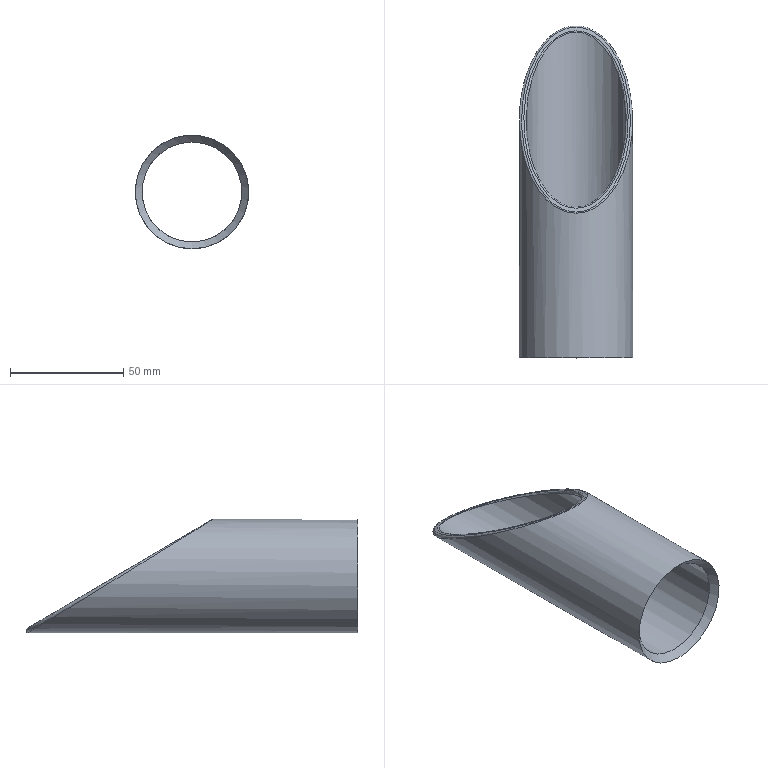Part | STEP file | JBJ-P-1004-05 | 1 solid | 6 faces | box 50 x 146.328 x 50 mm | volume 46289 mm3 | cylinder 2 | spline 2 | plane 1 | cone 1 | commonest cylinder face diameters 44 x1 50 x1
STEP:
#1=CARTESIAN_POINT('',(0.,1.,-25.));
#2=VERTEX_POINT('',#1);
#3=CARTESIAN_POINT('',(0.,1.,0.));
#4=DIRECTION('',(0.,1.,0.));
#5=DIRECTION('',(0.,0.,-1.));
#6=AXIS2_PLACEMENT_3D('',#3,#4,#5);
#7=CIRCLE('',#6,25.);
#8=EDGE_CURVE('',#2,#2,#7,.T.);
#9=ORIENTED_EDGE('',*,*,#8,.T.);
#10=EDGE_LOOP('',(#9));
#11=FACE_OUTER_BOUND('',#10,.T.);
#12=CARTESIAN_POINT('',(0.,64.728,25.));
#13=VERTEX_POINT('',#12);
#14=CARTESIAN_POINT('',(0.,64.728,25.));
#15=CARTESIAN_POINT('',(-50.,64.728,25.));
#16=CARTESIAN_POINT('',(-50.,146.328,-25.));
#17=CARTESIAN_POINT('',(0.,146.328,-25.));
#18=CARTESIAN_POINT('',(50.,146.328,-25.));
#19=CARTESIAN_POINT('',(50.,64.728,25.));
#20=CARTESIAN_POINT('',(0.,64.728,25.));
#21=(BOUNDED_CURVE()B_SPLINE_CURVE(3,(#14,#15,#16,#17,#18,#19,#20),.UNSPECIFIED.,.T.,.T.)B_SPLINE_CURVE_WITH_KNOTS((4,3,4),(0.,3.142,6.283),.UNSPECIFIED.)CURVE()GEOMETRIC_REPRESENTATION_ITEM()RATIONAL_B_SPLINE_CURVE((1.,0.3333,0.3333,1.,0.3333,0.3333,1.))REPRESENTATION_ITEM(''));
#22=EDGE_CURVE('',#13,#13,#21,.T.);
#23=ORIENTED_EDGE('',*,*,#22,.T.);
#24=EDGE_LOOP('',(#23));
#25=FACE_OUTER_BOUND('',#24,.T.);
#26=CARTESIAN_POINT('',(0.,150.,0.));
#27=DIRECTION('',(0.,-1.,0.));
#28=DIRECTION('',(0.,0.,-1.));
#29=AXIS2_PLACEMENT_3D('',#26,#27,#28);
#30=CYLINDRICAL_SURFACE('',#29,25.);
#31=ADVANCED_FACE('',(#11,#25),#30,.T.);
#32=CARTESIAN_POINT('',(0.,4.,22.));
#33=VERTEX_POINT('',#32);
#34=CARTESIAN_POINT('',(0.,4.,0.));
#35=DIRECTION('',(0.,-1.,0.));
#36=DIRECTION('',(0.,0.,1.));
#37=AXIS2_PLACEMENT_3D('',#34,#35,#36);
#38=CIRCLE('',#37,22.);
#39=EDGE_CURVE('',#33,#33,#38,.T.);
#40=ORIENTED_EDGE('',*,*,#39,.T.);
#41=EDGE_LOOP('',(#40));
#42=FACE_OUTER_BOUND('',#41,.T.);
#43=CARTESIAN_POINT('',(0.,66.428,22.));
#44=VERTEX_POINT('',#43);
#45=CARTESIAN_POINT('',(0.,66.428,22.));
#46=CARTESIAN_POINT('',(44.,66.428,22.));
#47=CARTESIAN_POINT('',(44.,144.628,-22.));
#48=CARTESIAN_POINT('',(0.,144.628,-22.));
#49=CARTESIAN_POINT('',(-44.,144.628,-22.));
#50=CARTESIAN_POINT('',(-44.,66.428,22.));
#51=CARTESIAN_POINT('',(0.,66.428,22.));
#52=(BOUNDED_CURVE()B_SPLINE_CURVE(3,(#45,#46,#47,#48,#49,#50,#51),.UNSPECIFIED.,.T.,.F.)B_SPLINE_CURVE_WITH_KNOTS((4,3,4),(0.,3.142,6.283),.UNSPECIFIED.)CURVE()GEOMETRIC_REPRESENTATION_ITEM()RATIONAL_B_SPLINE_CURVE((1.,0.3333,0.3333,1.,0.3333,0.3333,1.))REPRESENTATION_ITEM(''));
#53=EDGE_CURVE('',#44,#44,#52,.T.);
#54=ORIENTED_EDGE('',*,*,#53,.T.);
#55=EDGE_LOOP('',(#54));
#56=FACE_OUTER_BOUND('',#55,.T.);
#57=CARTESIAN_POINT('',(0.,150.,0.));
#58=DIRECTION('',(0.,-1.,0.));
#59=DIRECTION('',(0.,0.,-1.));
#60=AXIS2_PLACEMENT_3D('',#57,#58,#59);
#61=CYLINDRICAL_SURFACE('',#60,22.);
#62=ADVANCED_FACE('',(#42,#56),#61,.F.);
#63=CARTESIAN_POINT('',(0.,66.935,23.862));
#64=VERTEX_POINT('',#63);
#65=CARTESIAN_POINT('',(0.,66.935,23.862));
#66=CARTESIAN_POINT('',(-46.,66.935,23.862));
#67=CARTESIAN_POINT('',(-46.,145.135,-22.138));
#68=CARTESIAN_POINT('',(0.,145.135,-22.138));
#69=CARTESIAN_POINT('',(46.,145.135,-22.138));
#70=CARTESIAN_POINT('',(46.,66.935,23.862));
#71=CARTESIAN_POINT('',(0.,66.935,23.862));
#72=(BOUNDED_CURVE()B_SPLINE_CURVE(3,(#65,#66,#67,#68,#69,#70,#71),.UNSPECIFIED.,.T.,.F.)B_SPLINE_CURVE_WITH_KNOTS((4,3,4),(0.,3.142,6.283),.UNSPECIFIED.)CURVE()GEOMETRIC_REPRESENTATION_ITEM()RATIONAL_B_SPLINE_CURVE((1.,0.3333,0.3333,1.,0.3333,0.3333,1.))REPRESENTATION_ITEM(''));
#73=EDGE_CURVE('',#64,#64,#72,.T.);
#74=ORIENTED_EDGE('',*,*,#73,.T.);
#75=EDGE_LOOP('',(#74));
#76=FACE_BOUND('',#75,.T.);
#77=CARTESIAN_POINT('',(0.,65.235,24.862));
#78=VERTEX_POINT('',#77);
#79=CARTESIAN_POINT('',(0.,65.235,24.862));
#80=CARTESIAN_POINT('',(48.,65.235,24.862));
#81=CARTESIAN_POINT('',(48.,146.835,-23.138));
#82=CARTESIAN_POINT('',(0.,146.835,-23.138));
#83=CARTESIAN_POINT('',(-48.,146.835,-23.138));
#84=CARTESIAN_POINT('',(-48.,65.235,24.862));
#85=CARTESIAN_POINT('',(0.,65.235,24.862));
#86=(BOUNDED_CURVE()B_SPLINE_CURVE(3,(#79,#80,#81,#82,#83,#84,#85),.UNSPECIFIED.,.T.,.F.)B_SPLINE_CURVE_WITH_KNOTS((4,3,4),(0.,3.142,6.283),.UNSPECIFIED.)CURVE()GEOMETRIC_REPRESENTATION_ITEM()RATIONAL_B_SPLINE_CURVE((1.,0.3333,0.3333,1.,0.3333,0.3333,1.))REPRESENTATION_ITEM(''));
#87=EDGE_CURVE('',#78,#78,#86,.T.);
#88=ORIENTED_EDGE('',*,*,#87,.T.);
#89=EDGE_LOOP('',(#88));
#90=FACE_OUTER_BOUND('',#89,.T.);
#91=CARTESIAN_POINT('',(-25.,65.,25.));
#92=DIRECTION('',(0.,-0.507,-0.8619));
#93=DIRECTION('',(0.,0.8619,-0.507));
#94=AXIS2_PLACEMENT_3D('',#91,#92,#93);
#95=PLANE('',#94);
#96=ADVANCED_FACE('',(#76,#90),#95,.F.);
#97=ORIENTED_EDGE('',*,*,#53,.F.);
#98=EDGE_LOOP('',(#97));
#99=FACE_OUTER_BOUND('',#98,.T.);
#100=ORIENTED_EDGE('',*,*,#73,.F.);
#101=EDGE_LOOP('',(#100));
#102=FACE_OUTER_BOUND('',#101,.T.);
#103=CARTESIAN_POINT('',(0.,66.428,22.));
#104=CARTESIAN_POINT('',(0.,70.1,22.));
#105=CARTESIAN_POINT('',(0.,66.935,23.862));
#106=CARTESIAN_POINT('',(-0.7199,66.428,22.));
#107=CARTESIAN_POINT('',(-0.5156,70.1,22.));
#108=CARTESIAN_POINT('',(-0.7527,66.935,23.862));
#109=CARTESIAN_POINT('',(-1.44,66.491,21.965));
#110=CARTESIAN_POINT('',(-1.026,70.124,21.986));
#111=CARTESIAN_POINT('',(-1.505,66.998,23.825));
#112=CARTESIAN_POINT('',(-2.873,66.741,21.823));
#113=CARTESIAN_POINT('',(-2.093,70.237,21.92));
#114=CARTESIAN_POINT('',(-3.003,67.248,23.677));
#115=CARTESIAN_POINT('',(-3.586,66.929,21.718));
#116=CARTESIAN_POINT('',(-2.639,70.323,21.869));
#117=CARTESIAN_POINT('',(-3.749,67.436,23.567));
#118=CARTESIAN_POINT('',(-4.998,67.429,21.437));
#119=CARTESIAN_POINT('',(-3.791,70.589,21.713));
#120=CARTESIAN_POINT('',(-5.225,67.936,23.273));
#121=CARTESIAN_POINT('',(-5.697,67.74,21.262));
#122=CARTESIAN_POINT('',(-4.386,70.764,21.61));
#123=CARTESIAN_POINT('',(-5.956,68.247,23.09));
#124=CARTESIAN_POINT('',(-7.075,68.483,20.844));
#125=CARTESIAN_POINT('',(-5.624,71.236,21.332));
#126=CARTESIAN_POINT('',(-7.397,68.99,22.653));
#127=CARTESIAN_POINT('',(-7.754,68.914,20.601));
#128=CARTESIAN_POINT('',(-6.259,71.526,21.161));
#129=CARTESIAN_POINT('',(-8.106,69.421,22.399));
#130=CARTESIAN_POINT('',(-9.084,69.894,20.05));
#131=CARTESIAN_POINT('',(-7.553,72.242,20.74));
#132=CARTESIAN_POINT('',(-9.497,70.401,21.823));
#133=CARTESIAN_POINT('',(-9.736,70.441,19.742));
#134=CARTESIAN_POINT('',(-8.206,72.659,20.495));
#135=CARTESIAN_POINT('',(-10.178,70.948,21.501));
#136=CARTESIAN_POINT('',(-11.006,71.648,19.063));
#137=CARTESIAN_POINT('',(-9.512,73.631,19.923));
#138=CARTESIAN_POINT('',(-11.506,72.155,20.791));
#139=CARTESIAN_POINT('',(-11.624,72.306,18.692));
#140=CARTESIAN_POINT('',(-10.161,74.177,19.602));
#141=CARTESIAN_POINT('',(-12.152,72.813,20.404));
#142=CARTESIAN_POINT('',(-13.42,74.439,17.492));
#143=CARTESIAN_POINT('',(-12.027,75.966,18.549));
#144=CARTESIAN_POINT('',(-14.03,74.946,19.149));
#145=CARTESIAN_POINT('',(-14.538,76.07,16.575));
#146=CARTESIAN_POINT('',(-13.261,77.411,17.699));
#147=CARTESIAN_POINT('',(-15.199,76.577,18.19));
#148=CARTESIAN_POINT('',(-16.575,79.689,14.538));
#149=CARTESIAN_POINT('',(-15.529,80.774,15.721));
#150=CARTESIAN_POINT('',(-17.328,80.196,16.061));
#151=CARTESIAN_POINT('',(-17.492,81.677,13.42));
#152=CARTESIAN_POINT('',(-16.575,82.641,14.623));
#153=CARTESIAN_POINT('',(-18.287,82.184,14.892));
#154=CARTESIAN_POINT('',(-19.092,85.933,11.025));
#155=CARTESIAN_POINT('',(-18.399,86.73,12.218));
#156=CARTESIAN_POINT('',(-19.96,86.44,12.388));
#157=CARTESIAN_POINT('',(-19.774,88.2,9.749));
#158=CARTESIAN_POINT('',(-19.199,88.923,10.928));
#159=CARTESIAN_POINT('',(-20.673,88.707,11.054));
#160=CARTESIAN_POINT('',(-20.876,92.929,7.089));
#161=CARTESIAN_POINT('',(-20.492,93.54,8.211));
#162=CARTESIAN_POINT('',(-21.825,93.436,8.273));
#163=CARTESIAN_POINT('',(-21.296,95.39,5.704));
#164=CARTESIAN_POINT('',(-21.01,95.955,6.791));
#165=CARTESIAN_POINT('',(-22.264,95.897,6.825));
#166=CARTESIAN_POINT('',(-21.858,100.41,2.88));
#167=CARTESIAN_POINT('',(-21.724,100.899,3.883));
#168=CARTESIAN_POINT('',(-22.852,100.917,3.873));
#169=CARTESIAN_POINT('',(-22.,102.969,1.44));
#170=CARTESIAN_POINT('',(-21.942,103.431,2.394));
#171=CARTESIAN_POINT('',(-23.,103.476,2.367));
#172=CARTESIAN_POINT('',(-22.,108.087,-1.44));
#173=CARTESIAN_POINT('',(-22.055,108.496,-0.5858));
#174=CARTESIAN_POINT('',(-23.,108.594,-0.6434));
#175=CARTESIAN_POINT('',(-21.858,110.646,-2.88));
#176=CARTESIAN_POINT('',(-21.967,111.04,-2.082));
#177=CARTESIAN_POINT('',(-22.852,111.153,-2.149));
#178=CARTESIAN_POINT('',(-21.296,115.666,-5.704));
#179=CARTESIAN_POINT('',(-21.481,116.022,-5.013));
#180=CARTESIAN_POINT('',(-22.264,116.173,-5.102));
#181=CARTESIAN_POINT('',(-20.876,118.126,-7.089));
#182=CARTESIAN_POINT('',(-21.095,118.476,-6.456));
#183=CARTESIAN_POINT('',(-21.825,118.633,-6.549));
#184=CARTESIAN_POINT('',(-19.774,122.855,-9.749));
#185=CARTESIAN_POINT('',(-20.035,123.176,-9.221));
#186=CARTESIAN_POINT('',(-20.673,123.362,-9.331));
#187=CARTESIAN_POINT('',(-19.092,125.123,-11.025));
#188=CARTESIAN_POINT('',(-19.368,125.442,-10.554));
#189=CARTESIAN_POINT('',(-19.96,125.63,-10.665));
#190=CARTESIAN_POINT('',(-17.492,129.378,-13.42));
#191=CARTESIAN_POINT('',(-17.78,129.677,-13.045));
#192=CARTESIAN_POINT('',(-18.287,129.885,-13.168));
#193=CARTESIAN_POINT('',(-16.575,131.366,-14.538));
#194=CARTESIAN_POINT('',(-16.862,131.666,-14.215));
#195=CARTESIAN_POINT('',(-17.328,131.873,-14.337));
#196=CARTESIAN_POINT('',(-14.538,134.985,-16.575));
#197=CARTESIAN_POINT('',(-14.812,135.27,-16.335));
#198=CARTESIAN_POINT('',(-15.199,135.492,-16.466));
#199=CARTESIAN_POINT('',(-13.42,136.616,-17.492));
#200=CARTESIAN_POINT('',(-13.68,136.904,-17.297));
#201=CARTESIAN_POINT('',(-14.03,137.123,-17.426));
#202=CARTESIAN_POINT('',(-11.025,139.46,-19.092));
#203=CARTESIAN_POINT('',(-11.251,139.737,-18.963));
#204=CARTESIAN_POINT('',(-11.526,139.967,-19.098));
#205=CARTESIAN_POINT('',(-9.749,140.672,-19.774));
#206=CARTESIAN_POINT('',(-9.951,140.952,-19.678));
#207=CARTESIAN_POINT('',(-10.192,141.179,-19.811));
#208=CARTESIAN_POINT('',(-7.089,142.631,-20.876));
#209=CARTESIAN_POINT('',(-7.242,142.904,-20.826));
#210=CARTESIAN_POINT('',(-7.411,143.138,-20.963));
#211=CARTESIAN_POINT('',(-5.704,143.377,-21.296));
#212=CARTESIAN_POINT('',(-5.827,143.652,-21.266));
#213=CARTESIAN_POINT('',(-5.963,143.884,-21.402));
#214=CARTESIAN_POINT('',(-2.88,144.376,-21.858));
#215=CARTESIAN_POINT('',(-2.945,144.647,-21.851));
#216=CARTESIAN_POINT('',(-3.011,144.883,-21.99));
#217=CARTESIAN_POINT('',(-1.44,144.628,-22.));
#218=CARTESIAN_POINT('',(-1.47,144.9,-22.));
#219=CARTESIAN_POINT('',(-1.505,145.135,-22.138));
#220=CARTESIAN_POINT('',(1.44,144.628,-22.));
#221=CARTESIAN_POINT('',(1.47,144.9,-22.));
#222=CARTESIAN_POINT('',(1.505,145.135,-22.138));
#223=CARTESIAN_POINT('',(2.88,144.376,-21.858));
#224=CARTESIAN_POINT('',(2.945,144.647,-21.851));
#225=CARTESIAN_POINT('',(3.011,144.883,-21.99));
#226=CARTESIAN_POINT('',(5.704,143.377,-21.296));
#227=CARTESIAN_POINT('',(5.827,143.652,-21.266));
#228=CARTESIAN_POINT('',(5.963,143.884,-21.402));
#229=CARTESIAN_POINT('',(7.089,142.631,-20.876));
#230=CARTESIAN_POINT('',(7.242,142.904,-20.826));
#231=CARTESIAN_POINT('',(7.411,143.138,-20.963));
#232=CARTESIAN_POINT('',(9.749,140.672,-19.774));
#233=CARTESIAN_POINT('',(9.951,140.952,-19.678));
#234=CARTESIAN_POINT('',(10.192,141.179,-19.811));
#235=CARTESIAN_POINT('',(11.025,139.46,-19.092));
#236=CARTESIAN_POINT('',(11.251,139.737,-18.963));
#237=CARTESIAN_POINT('',(11.526,139.967,-19.098));
#238=CARTESIAN_POINT('',(13.42,136.616,-17.492));
#239=CARTESIAN_POINT('',(13.68,136.904,-17.297));
#240=CARTESIAN_POINT('',(14.03,137.123,-17.426));
#241=CARTESIAN_POINT('',(14.538,134.985,-16.575));
#242=CARTESIAN_POINT('',(14.812,135.27,-16.335));
#243=CARTESIAN_POINT('',(15.199,135.492,-16.466));
#244=CARTESIAN_POINT('',(16.575,131.366,-14.538));
#245=CARTESIAN_POINT('',(16.862,131.666,-14.215));
#246=CARTESIAN_POINT('',(17.328,131.873,-14.337));
#247=CARTESIAN_POINT('',(17.492,129.378,-13.42));
#248=CARTESIAN_POINT('',(17.78,129.677,-13.045));
#249=CARTESIAN_POINT('',(18.287,129.885,-13.168));
#250=CARTESIAN_POINT('',(19.092,125.123,-11.025));
#251=CARTESIAN_POINT('',(19.368,125.442,-10.554));
#252=CARTESIAN_POINT('',(19.96,125.63,-10.665));
#253=CARTESIAN_POINT('',(19.774,122.855,-9.749));
#254=CARTESIAN_POINT('',(20.035,123.176,-9.221));
#255=CARTESIAN_POINT('',(20.673,123.362,-9.331));
#256=CARTESIAN_POINT('',(20.876,118.126,-7.089));
#257=CARTESIAN_POINT('',(21.095,118.476,-6.456));
#258=CARTESIAN_POINT('',(21.825,118.633,-6.549));
#259=CARTESIAN_POINT('',(21.296,115.666,-5.704));
#260=CARTESIAN_POINT('',(21.481,116.022,-5.013));
#261=CARTESIAN_POINT('',(22.264,116.173,-5.102));
#262=CARTESIAN_POINT('',(21.858,110.646,-2.88));
#263=CARTESIAN_POINT('',(21.967,111.04,-2.082));
#264=CARTESIAN_POINT('',(22.852,111.153,-2.149));
#265=CARTESIAN_POINT('',(22.,108.087,-1.44));
#266=CARTESIAN_POINT('',(22.055,108.496,-0.5858));
#267=CARTESIAN_POINT('',(23.,108.594,-0.6434));
#268=CARTESIAN_POINT('',(22.,102.969,1.44));
#269=CARTESIAN_POINT('',(21.942,103.431,2.394));
#270=CARTESIAN_POINT('',(23.,103.476,2.367));
#271=CARTESIAN_POINT('',(21.858,100.41,2.88));
#272=CARTESIAN_POINT('',(21.724,100.899,3.883));
#273=CARTESIAN_POINT('',(22.852,100.917,3.873));
#274=CARTESIAN_POINT('',(21.296,95.39,5.704));
#275=CARTESIAN_POINT('',(21.01,95.955,6.791));
#276=CARTESIAN_POINT('',(22.264,95.897,6.825));
#277=CARTESIAN_POINT('',(20.876,92.929,7.089));
#278=CARTESIAN_POINT('',(20.492,93.54,8.211));
#279=CARTESIAN_POINT('',(21.825,93.436,8.273));
#280=CARTESIAN_POINT('',(19.774,88.2,9.749));
#281=CARTESIAN_POINT('',(19.199,88.923,10.928));
#282=CARTESIAN_POINT('',(20.673,88.707,11.054));
#283=CARTESIAN_POINT('',(19.092,85.933,11.025));
#284=CARTESIAN_POINT('',(18.399,86.73,12.218));
#285=CARTESIAN_POINT('',(19.96,86.44,12.388));
#286=CARTESIAN_POINT('',(17.492,81.677,13.42));
#287=CARTESIAN_POINT('',(16.575,82.641,14.623));
#288=CARTESIAN_POINT('',(18.287,82.184,14.892));
#289=CARTESIAN_POINT('',(16.575,79.689,14.538));
#290=CARTESIAN_POINT('',(15.529,80.774,15.721));
#291=CARTESIAN_POINT('',(17.328,80.196,16.061));
#292=CARTESIAN_POINT('',(14.538,76.07,16.575));
#293=CARTESIAN_POINT('',(13.261,77.411,17.699));
#294=CARTESIAN_POINT('',(15.199,76.577,18.19));
#295=CARTESIAN_POINT('',(13.42,74.439,17.492));
#296=CARTESIAN_POINT('',(12.027,75.966,18.549));
#297=CARTESIAN_POINT('',(14.03,74.946,19.149));
#298=CARTESIAN_POINT('',(11.624,72.306,18.692));
#299=CARTESIAN_POINT('',(10.161,74.177,19.602));
#300=CARTESIAN_POINT('',(12.152,72.813,20.404));
#301=CARTESIAN_POINT('',(11.006,71.648,19.063));
#302=CARTESIAN_POINT('',(9.512,73.631,19.923));
#303=CARTESIAN_POINT('',(11.506,72.155,20.791));
#304=CARTESIAN_POINT('',(9.736,70.441,19.742));
#305=CARTESIAN_POINT('',(8.206,72.659,20.495));
#306=CARTESIAN_POINT('',(10.178,70.948,21.501));
#307=CARTESIAN_POINT('',(9.084,69.894,20.05));
#308=CARTESIAN_POINT('',(7.553,72.242,20.74));
#309=CARTESIAN_POINT('',(9.497,70.401,21.823));
#310=CARTESIAN_POINT('',(7.754,68.914,20.601));
#311=CARTESIAN_POINT('',(6.259,71.526,21.161));
#312=CARTESIAN_POINT('',(8.106,69.421,22.399));
#313=CARTESIAN_POINT('',(7.075,68.483,20.844));
#314=CARTESIAN_POINT('',(5.624,71.236,21.332));
#315=CARTESIAN_POINT('',(7.397,68.99,22.653));
#316=CARTESIAN_POINT('',(5.697,67.74,21.262));
#317=CARTESIAN_POINT('',(4.386,70.764,21.61));
#318=CARTESIAN_POINT('',(5.956,68.247,23.09));
#319=CARTESIAN_POINT('',(4.998,67.429,21.437));
#320=CARTESIAN_POINT('',(3.791,70.589,21.713));
#321=CARTESIAN_POINT('',(5.225,67.936,23.273));
#322=CARTESIAN_POINT('',(3.586,66.929,21.718));
#323=CARTESIAN_POINT('',(2.639,70.323,21.869));
#324=CARTESIAN_POINT('',(3.749,67.436,23.567));
#325=CARTESIAN_POINT('',(2.873,66.741,21.823));
#326=CARTESIAN_POINT('',(2.093,70.237,21.92));
#327=CARTESIAN_POINT('',(3.003,67.248,23.677));
#328=CARTESIAN_POINT('',(1.44,66.491,21.965));
#329=CARTESIAN_POINT('',(1.026,70.124,21.986));
#330=CARTESIAN_POINT('',(1.505,66.998,23.825));
#331=CARTESIAN_POINT('',(0.7199,66.428,22.));
#332=CARTESIAN_POINT('',(0.5156,70.1,22.));
#333=CARTESIAN_POINT('',(0.7527,66.935,23.862));
#334=CARTESIAN_POINT('',(0.,66.428,22.));
#335=CARTESIAN_POINT('',(0.,70.1,22.));
#336=CARTESIAN_POINT('',(0.,66.935,23.862));
#337=(BOUNDED_SURFACE()B_SPLINE_SURFACE(3,2,((#103,#104,#105),(#106,#107,#108),(#109,#110,#111),(#112,#113,#114),(#115,#116,#117),(#118,#119,#120),(#121,#122,#123),(#124,#125,#126),(#127,#128,#129),(#130,#131,#132),(#133,#134,#135),(#136,#137,#138),(#139,#140,#141),(#142,#143,#144),(#145,#146,#147),(#148,#149,#150),(#151,#152,#153),(#154,#155,#156),(#157,#158,#159),(#160,#161,#162),(#163,#164,#165),(#166,#167,#168),(#169,#170,#171),(#172,#173,#174),(#175,#176,#177),(#178,#179,#180),(#181,#182,#183),(#184,#185,#186),(#187,#188,#189),(#190,#191,#192),(#193,#194,#195),(#196,#197,#198),(#199,#200,#201),(#202,#203,#204),(#205,#206,#207),(#208,#209,#210),(#211,#212,#213),(#214,#215,#216),(#217,#218,#219),(#220,#221,#222),(#223,#224,#225),(#226,#227,#228),(#229,#230,#231),(#232,#233,#234),(#235,#236,#237),(#238,#239,#240),(#241,#242,#243),(#244,#245,#246),(#247,#248,#249),(#250,#251,#252),(#253,#254,#255),(#256,#257,#258),(#259,#260,#261),(#262,#263,#264),(#265,#266,#267),(#268,#269,#270),(#271,#272,#273),(#274,#275,#276),(#277,#278,#279),(#280,#281,#282),(#283,#284,#285),(#286,#287,#288),(#289,#290,#291),(#292,#293,#294),(#295,#296,#297),(#298,#299,#300),(#301,#302,#303),(#304,#305,#306),(#307,#308,#309),(#310,#311,#312),(#313,#314,#315),(#316,#317,#318),(#319,#320,#321),(#322,#323,#324),(#325,#326,#327),(#328,#329,#330),(#331,#332,#333),(#334,#335,#336)),.UNSPECIFIED.,.T.,.F.,.F.)B_SPLINE_SURFACE_WITH_KNOTS((4,2,2,2,2,2,2,2,2,2,2,2,2,2,2,2,2,2,2,2,2,2,2,2,2,2,2,2,2,2,2,2,2,2,2,2,2,2,4),(3,3),(0.,0.09817,0.1963,0.2945,0.3927,0.4909,0.589,0.7854,0.9817,1.178,1.374,1.571,1.767,1.963,2.16,2.356,2.553,2.749,2.945,3.142,3.338,3.534,3.731,3.927,4.123,4.32,4.516,4.712,4.909,5.105,5.301,5.498,5.694,5.792,5.89,5.989,6.087,6.185,6.283),(0.,1.),.UNSPECIFIED.)GEOMETRIC_REPRESENTATION_ITEM()RATIONAL_B_SPLINE_SURFACE(((1.,0.2627,1.),(1.,0.2627,1.),(1.,0.2641,1.),(1.,0.2693,1.),(1.,0.2731,1.),(1.,0.283,1.),(1.,0.289,1.),(1.,0.3029,1.),(1.,0.3107,1.),(1.,0.3276,1.),(1.,0.3367,1.),(1.,0.3559,1.),(1.,0.366,1.),(1.,0.3972,1.),(1.,0.4193,1.),(1.,0.4645,1.),(1.,0.4875,1.),(1.,0.5334,1.),(1.,0.5563,1.),(1.,0.6014,1.),(1.,0.6235,1.),(1.,0.6664,1.),(1.,0.6872,1.),(1.,0.7271,1.),(1.,0.7462,1.),(1.,0.7823,1.),(1.,0.7994,1.),(1.,0.8314,1.),(1.,0.8463,1.),(1.,0.8735,1.),(1.,0.886,1.),(1.,0.9082,1.),(1.,0.918,1.),(1.,0.9349,1.),(1.,0.942,1.),(1.,0.9534,1.),(1.,0.9577,1.),(1.,0.9634,1.),(1.,0.9649,1.),(1.,0.9649,1.),(1.,0.9634,1.),(1.,0.9577,1.),(1.,0.9534,1.),(1.,0.942,1.),(1.,0.9349,1.),(1.,0.918,1.),(1.,0.9082,1.),(1.,0.886,1.),(1.,0.8735,1.),(1.,0.8463,1.),(1.,0.8314,1.),(1.,0.7994,1.),(1.,0.7823,1.),(1.,0.7462,1.),(1.,0.7271,1.),(1.,0.6872,1.),(1.,0.6664,1.),(1.,0.6235,1.),(1.,0.6014,1.),(1.,0.5563,1.),(1.,0.5334,1.),(1.,0.4875,1.),(1.,0.4645,1.),(1.,0.4193,1.),(1.,0.3972,1.),(1.,0.366,1.),(1.,0.3559,1.),(1.,0.3367,1.),(1.,0.3276,1.),(1.,0.3107,1.),(1.,0.3029,1.),(1.,0.289,1.),(1.,0.283,1.),(1.,0.2731,1.),(1.,0.2693,1.),(1.,0.2641,1.),(1.,0.2627,1.),(1.,0.2627,1.)))REPRESENTATION_ITEM('')SURFACE());
#338=ADVANCED_FACE('',(#99,#102),#337,.T.);
#339=ORIENTED_EDGE('',*,*,#87,.F.);
#340=EDGE_LOOP('',(#339));
#341=FACE_OUTER_BOUND('',#340,.T.);
#342=ORIENTED_EDGE('',*,*,#22,.F.);
#343=EDGE_LOOP('',(#342));
#344=FACE_OUTER_BOUND('',#343,.T.);
#345=CARTESIAN_POINT('',(0.,65.235,24.862));
#346=CARTESIAN_POINT('',(0.,65.,25.));
#347=CARTESIAN_POINT('',(0.,64.728,25.));
#348=CARTESIAN_POINT('',(-1.571,65.235,24.862));
#349=CARTESIAN_POINT('',(-1.606,65.,25.));
#350=CARTESIAN_POINT('',(-1.636,64.728,25.));
#351=CARTESIAN_POINT('',(-3.142,65.498,24.707));
#352=CARTESIAN_POINT('',(-3.217,65.265,24.844));
#353=CARTESIAN_POINT('',(-3.272,64.991,24.839));
#354=CARTESIAN_POINT('',(-6.223,66.54,24.094));
#355=CARTESIAN_POINT('',(-6.369,66.311,24.229));
#356=CARTESIAN_POINT('',(-6.482,66.033,24.2));
#357=CARTESIAN_POINT('',(-7.733,67.319,23.636));
#358=CARTESIAN_POINT('',(-7.919,67.096,23.767));
#359=CARTESIAN_POINT('',(-8.055,66.812,23.723));
#360=CARTESIAN_POINT('',(-10.636,69.362,22.434));
#361=CARTESIAN_POINT('',(-10.894,69.147,22.56));
#362=CARTESIAN_POINT('',(-11.079,68.855,22.471));
#363=CARTESIAN_POINT('',(-12.028,70.627,21.69));
#364=CARTESIAN_POINT('',(-12.326,70.424,21.81));
#365=CARTESIAN_POINT('',(-12.529,70.12,21.696));
#366=CARTESIAN_POINT('',(-14.64,73.594,19.945));
#367=CARTESIAN_POINT('',(-15.013,73.402,20.058));
#368=CARTESIAN_POINT('',(-15.25,73.087,19.878));
#369=CARTESIAN_POINT('',(-15.86,75.297,18.943));
#370=CARTESIAN_POINT('',(-16.274,75.12,19.047));
#371=CARTESIAN_POINT('',(-16.521,74.79,18.835));
#372=CARTESIAN_POINT('',(-18.081,79.073,16.722));
#373=CARTESIAN_POINT('',(-18.575,78.913,16.816));
#374=CARTESIAN_POINT('',(-18.835,78.566,16.521));
#375=CARTESIAN_POINT('',(-19.083,81.147,15.502));
#376=CARTESIAN_POINT('',(-19.617,81.007,15.584));
#377=CARTESIAN_POINT('',(-19.878,80.64,15.25));
#378=CARTESIAN_POINT('',(-20.828,85.588,12.89));
#379=CARTESIAN_POINT('',(-21.447,85.47,12.959));
#380=CARTESIAN_POINT('',(-21.696,85.081,12.529));
#381=CARTESIAN_POINT('',(-21.572,87.954,11.498));
#382=CARTESIAN_POINT('',(-22.233,87.861,11.552));
#383=CARTESIAN_POINT('',(-22.471,87.447,11.079));
#384=CARTESIAN_POINT('',(-22.774,92.888,8.595));
#385=CARTESIAN_POINT('',(-23.528,92.827,8.631));
#386=CARTESIAN_POINT('',(-23.723,92.381,8.055));
#387=CARTESIAN_POINT('',(-23.232,95.456,7.085));
#388=CARTESIAN_POINT('',(-24.03,95.424,7.104));
#389=CARTESIAN_POINT('',(-24.2,94.949,6.482));
#390=CARTESIAN_POINT('',(-23.845,100.694,4.003));
#391=CARTESIAN_POINT('',(-24.744,100.706,3.997));
#392=CARTESIAN_POINT('',(-24.839,100.187,3.272));
#393=CARTESIAN_POINT('',(-24.,103.364,2.433));
#394=CARTESIAN_POINT('',(-24.945,103.41,2.406));
#395=CARTESIAN_POINT('',(-25.,102.857,1.636));
#396=CARTESIAN_POINT('',(-24.,108.705,-0.7089));
#397=CARTESIAN_POINT('',(-25.058,108.812,-0.7718));
#398=CARTESIAN_POINT('',(-25.,108.198,-1.636));
#399=CARTESIAN_POINT('',(-23.845,111.375,-2.28));
#400=CARTESIAN_POINT('',(-24.953,111.523,-2.366));
#401=CARTESIAN_POINT('',(-24.839,110.868,-3.272));
#402=CARTESIAN_POINT('',(-23.232,116.613,-5.361));
#403=CARTESIAN_POINT('',(-24.466,116.848,-5.499));
#404=CARTESIAN_POINT('',(-24.2,116.106,-6.482));
#405=CARTESIAN_POINT('',(-22.774,119.181,-6.871));
#406=CARTESIAN_POINT('',(-24.063,119.466,-7.039));
#407=CARTESIAN_POINT('',(-23.723,118.674,-8.055));
#408=CARTESIAN_POINT('',(-21.572,124.115,-9.774));
#409=CARTESIAN_POINT('',(-22.999,124.526,-10.015));
#410=CARTESIAN_POINT('',(-22.471,123.608,-11.079));
#411=CARTESIAN_POINT('',(-20.828,126.482,-11.166));
#412=CARTESIAN_POINT('',(-22.315,126.959,-11.447));
#413=CARTESIAN_POINT('',(-21.696,125.975,-12.529));
#414=CARTESIAN_POINT('',(-19.083,130.922,-13.778));
#415=CARTESIAN_POINT('',(-20.714,131.585,-14.167));
#416=CARTESIAN_POINT('',(-19.878,130.415,-15.25));
#417=CARTESIAN_POINT('',(-18.081,132.996,-14.998));
#418=CARTESIAN_POINT('',(-19.775,133.753,-15.443));
#419=CARTESIAN_POINT('',(-18.835,132.489,-16.521));
#420=CARTESIAN_POINT('',(-15.86,136.773,-17.219));
#421=CARTESIAN_POINT('',(-17.681,137.806,-17.827));
#422=CARTESIAN_POINT('',(-16.521,136.266,-18.835));
#423=CARTESIAN_POINT('',(-14.64,138.475,-18.221));
#424=CARTESIAN_POINT('',(-16.509,139.648,-18.91));
#425=CARTESIAN_POINT('',(-15.25,137.968,-19.878));
#426=CARTESIAN_POINT('',(-12.028,141.442,-19.966));
#427=CARTESIAN_POINT('',(-13.938,143.021,-20.895));
#428=CARTESIAN_POINT('',(-12.529,140.935,-21.696));
#429=CARTESIAN_POINT('',(-10.636,142.707,-20.71));
#430=CARTESIAN_POINT('',(-12.534,144.49,-21.759));
#431=CARTESIAN_POINT('',(-11.079,142.2,-22.471));
#432=CARTESIAN_POINT('',(-8.459,144.24,-21.612));
#433=CARTESIAN_POINT('',(-10.268,146.372,-22.866));
#434=CARTESIAN_POINT('',(-8.811,143.733,-23.41));
#435=CARTESIAN_POINT('',(-7.718,144.69,-21.877));
#436=CARTESIAN_POINT('',(-9.457,146.954,-23.208));
#437=CARTESIAN_POINT('',(-8.04,144.183,-23.686));
#438=CARTESIAN_POINT('',(-6.215,145.465,-22.333));
#439=CARTESIAN_POINT('',(-7.751,148.001,-23.824));
#440=CARTESIAN_POINT('',(-6.474,144.958,-24.161));
#441=CARTESIAN_POINT('',(-5.452,145.79,-22.524));
#442=CARTESIAN_POINT('',(-6.861,148.452,-24.089));
#443=CARTESIAN_POINT('',(-5.68,145.283,-24.36));
#444=CARTESIAN_POINT('',(-3.912,146.311,-22.83));
#445=CARTESIAN_POINT('',(-4.994,149.207,-24.533));
#446=CARTESIAN_POINT('',(-4.075,145.804,-24.679));
#447=CARTESIAN_POINT('',(-3.134,146.507,-22.946));
#448=CARTESIAN_POINT('',(-4.029,149.498,-24.705));
#449=CARTESIAN_POINT('',(-3.265,146.,-24.799));
#450=CARTESIAN_POINT('',(-1.571,146.769,-23.099));
#451=CARTESIAN_POINT('',(-2.035,149.899,-24.94));
#452=CARTESIAN_POINT('',(-1.636,146.262,-24.96));
#453=CARTESIAN_POINT('',(-0.7854,146.835,-23.138));
#454=CARTESIAN_POINT('',(-1.022,150.,-25.));
#455=CARTESIAN_POINT('',(-0.8181,146.328,-25.));
#456=CARTESIAN_POINT('',(0.7854,146.835,-23.138));
#457=CARTESIAN_POINT('',(1.022,150.,-25.));
#458=CARTESIAN_POINT('',(0.8181,146.328,-25.));
#459=CARTESIAN_POINT('',(1.571,146.769,-23.099));
#460=CARTESIAN_POINT('',(2.035,149.899,-24.94));
#461=CARTESIAN_POINT('',(1.636,146.262,-24.96));
#462=CARTESIAN_POINT('',(3.134,146.507,-22.946));
#463=CARTESIAN_POINT('',(4.029,149.498,-24.705));
#464=CARTESIAN_POINT('',(3.265,146.,-24.799));
#465=CARTESIAN_POINT('',(3.912,146.311,-22.83));
#466=CARTESIAN_POINT('',(4.994,149.207,-24.533));
#467=CARTESIAN_POINT('',(4.075,145.804,-24.679));
#468=CARTESIAN_POINT('',(5.452,145.79,-22.524));
#469=CARTESIAN_POINT('',(6.861,148.452,-24.089));
#470=CARTESIAN_POINT('',(5.68,145.283,-24.36));
#471=CARTESIAN_POINT('',(6.215,145.465,-22.333));
#472=CARTESIAN_POINT('',(7.751,148.001,-23.824));
#473=CARTESIAN_POINT('',(6.474,144.958,-24.161));
#474=CARTESIAN_POINT('',(7.718,144.69,-21.877));
#475=CARTESIAN_POINT('',(9.457,146.954,-23.208));
#476=CARTESIAN_POINT('',(8.04,144.183,-23.686));
#477=CARTESIAN_POINT('',(8.459,144.24,-21.612));
#478=CARTESIAN_POINT('',(10.268,146.372,-22.866));
#479=CARTESIAN_POINT('',(8.811,143.733,-23.41));
#480=CARTESIAN_POINT('',(10.636,142.707,-20.71));
#481=CARTESIAN_POINT('',(12.534,144.49,-21.759));
#482=CARTESIAN_POINT('',(11.079,142.2,-22.471));
#483=CARTESIAN_POINT('',(12.028,141.442,-19.966));
#484=CARTESIAN_POINT('',(13.938,143.021,-20.895));
#485=CARTESIAN_POINT('',(12.529,140.935,-21.696));
#486=CARTESIAN_POINT('',(14.64,138.475,-18.221));
#487=CARTESIAN_POINT('',(16.509,139.648,-18.91));
#488=CARTESIAN_POINT('',(15.25,137.968,-19.878));
#489=CARTESIAN_POINT('',(15.86,136.773,-17.219));
#490=CARTESIAN_POINT('',(17.681,137.806,-17.827));
#491=CARTESIAN_POINT('',(16.521,136.266,-18.835));
#492=CARTESIAN_POINT('',(18.081,132.996,-14.998));
#493=CARTESIAN_POINT('',(19.775,133.753,-15.443));
#494=CARTESIAN_POINT('',(18.835,132.489,-16.521));
#495=CARTESIAN_POINT('',(19.083,130.922,-13.778));
#496=CARTESIAN_POINT('',(20.714,131.585,-14.167));
#497=CARTESIAN_POINT('',(19.878,130.415,-15.25));
#498=CARTESIAN_POINT('',(20.828,126.482,-11.166));
#499=CARTESIAN_POINT('',(22.315,126.959,-11.447));
#500=CARTESIAN_POINT('',(21.696,125.975,-12.529));
#501=CARTESIAN_POINT('',(21.572,124.115,-9.774));
#502=CARTESIAN_POINT('',(22.999,124.526,-10.015));
#503=CARTESIAN_POINT('',(22.471,123.608,-11.079));
#504=CARTESIAN_POINT('',(22.774,119.181,-6.871));
#505=CARTESIAN_POINT('',(24.063,119.466,-7.039));
#506=CARTESIAN_POINT('',(23.723,118.674,-8.055));
#507=CARTESIAN_POINT('',(23.232,116.613,-5.361));
#508=CARTESIAN_POINT('',(24.466,116.848,-5.499));
#509=CARTESIAN_POINT('',(24.2,116.106,-6.482));
#510=CARTESIAN_POINT('',(23.845,111.375,-2.28));
#511=CARTESIAN_POINT('',(24.953,111.523,-2.366));
#512=CARTESIAN_POINT('',(24.839,110.868,-3.272));
#513=CARTESIAN_POINT('',(24.,108.705,-0.7089));
#514=CARTESIAN_POINT('',(25.058,108.812,-0.7718));
#515=CARTESIAN_POINT('',(25.,108.198,-1.636));
#516=CARTESIAN_POINT('',(24.,103.364,2.433));
#517=CARTESIAN_POINT('',(24.945,103.41,2.406));
#518=CARTESIAN_POINT('',(25.,102.857,1.636));
#519=CARTESIAN_POINT('',(23.845,100.694,4.003));
#520=CARTESIAN_POINT('',(24.744,100.706,3.997));
#521=CARTESIAN_POINT('',(24.839,100.187,3.272));
#522=CARTESIAN_POINT('',(23.232,95.456,7.085));
#523=CARTESIAN_POINT('',(24.03,95.424,7.104));
#524=CARTESIAN_POINT('',(24.2,94.949,6.482));
#525=CARTESIAN_POINT('',(22.774,92.888,8.595));
#526=CARTESIAN_POINT('',(23.528,92.827,8.631));
#527=CARTESIAN_POINT('',(23.723,92.381,8.055));
#528=CARTESIAN_POINT('',(21.572,87.954,11.498));
#529=CARTESIAN_POINT('',(22.233,87.861,11.552));
#530=CARTESIAN_POINT('',(22.471,87.447,11.079));
#531=CARTESIAN_POINT('',(20.828,85.588,12.89));
#532=CARTESIAN_POINT('',(21.447,85.47,12.959));
#533=CARTESIAN_POINT('',(21.696,85.081,12.529));
#534=CARTESIAN_POINT('',(19.083,81.147,15.502));
#535=CARTESIAN_POINT('',(19.617,81.007,15.584));
#536=CARTESIAN_POINT('',(19.878,80.64,15.25));
#537=CARTESIAN_POINT('',(18.081,79.073,16.722));
#538=CARTESIAN_POINT('',(18.575,78.913,16.816));
#539=CARTESIAN_POINT('',(18.835,78.566,16.521));
#540=CARTESIAN_POINT('',(15.86,75.297,18.943));
#541=CARTESIAN_POINT('',(16.274,75.12,19.047));
#542=CARTESIAN_POINT('',(16.521,74.79,18.835));
#543=CARTESIAN_POINT('',(14.64,73.594,19.945));
#544=CARTESIAN_POINT('',(15.013,73.402,20.058));
#545=CARTESIAN_POINT('',(15.25,73.087,19.878));
#546=CARTESIAN_POINT('',(12.028,70.627,21.69));
#547=CARTESIAN_POINT('',(12.326,70.424,21.81));
#548=CARTESIAN_POINT('',(12.529,70.12,21.696));
#549=CARTESIAN_POINT('',(10.636,69.362,22.434));
#550=CARTESIAN_POINT('',(10.894,69.147,22.56));
#551=CARTESIAN_POINT('',(11.079,68.855,22.471));
#552=CARTESIAN_POINT('',(7.733,67.319,23.636));
#553=CARTESIAN_POINT('',(7.919,67.096,23.767));
#554=CARTESIAN_POINT('',(8.055,66.812,23.723));
#555=CARTESIAN_POINT('',(6.223,66.54,24.094));
#556=CARTESIAN_POINT('',(6.369,66.311,24.229));
#557=CARTESIAN_POINT('',(6.482,66.033,24.2));
#558=CARTESIAN_POINT('',(3.142,65.498,24.707));
#559=CARTESIAN_POINT('',(3.217,65.265,24.844));
#560=CARTESIAN_POINT('',(3.272,64.991,24.839));
#561=CARTESIAN_POINT('',(1.571,65.235,24.862));
#562=CARTESIAN_POINT('',(1.606,65.,25.));
#563=CARTESIAN_POINT('',(1.636,64.728,25.));
#564=CARTESIAN_POINT('',(0.,65.235,24.862));
#565=CARTESIAN_POINT('',(0.,65.,25.));
#566=CARTESIAN_POINT('',(0.,64.728,25.));
#567=(BOUNDED_SURFACE()B_SPLINE_SURFACE(3,2,((#345,#346,#347),(#348,#349,#350),(#351,#352,#353),(#354,#355,#356),(#357,#358,#359),(#360,#361,#362),(#363,#364,#365),(#366,#367,#368),(#369,#370,#371),(#372,#373,#374),(#375,#376,#377),(#378,#379,#380),(#381,#382,#383),(#384,#385,#386),(#387,#388,#389),(#390,#391,#392),(#393,#394,#395),(#396,#397,#398),(#399,#400,#401),(#402,#403,#404),(#405,#406,#407),(#408,#409,#410),(#411,#412,#413),(#414,#415,#416),(#417,#418,#419),(#420,#421,#422),(#423,#424,#425),(#426,#427,#428),(#429,#430,#431),(#432,#433,#434),(#435,#436,#437),(#438,#439,#440),(#441,#442,#443),(#444,#445,#446),(#447,#448,#449),(#450,#451,#452),(#453,#454,#455),(#456,#457,#458),(#459,#460,#461),(#462,#463,#464),(#465,#466,#467),(#468,#469,#470),(#471,#472,#473),(#474,#475,#476),(#477,#478,#479),(#480,#481,#482),(#483,#484,#485),(#486,#487,#488),(#489,#490,#491),(#492,#493,#494),(#495,#496,#497),(#498,#499,#500),(#501,#502,#503),(#504,#505,#506),(#507,#508,#509),(#510,#511,#512),(#513,#514,#515),(#516,#517,#518),(#519,#520,#521),(#522,#523,#524),(#525,#526,#527),(#528,#529,#530),(#531,#532,#533),(#534,#535,#536),(#537,#538,#539),(#540,#541,#542),(#543,#544,#545),(#546,#547,#548),(#549,#550,#551),(#552,#553,#554),(#555,#556,#557),(#558,#559,#560),(#561,#562,#563),(#564,#565,#566)),.UNSPECIFIED.,.T.,.F.,.T.)B_SPLINE_SURFACE_WITH_KNOTS((4,2,2,2,2,2,2,2,2,2,2,2,2,2,2,2,2,2,2,2,2,2,2,2,2,2,2,2,2,2,2,2,2,2,2,2,4),(3,3),(0.,0.1963,0.3927,0.589,0.7854,0.9817,1.178,1.374,1.571,1.767,1.963,2.16,2.356,2.553,2.749,2.847,2.945,3.043,3.142,3.24,3.338,3.436,3.534,3.731,3.927,4.123,4.32,4.516,4.712,4.909,5.105,5.301,5.498,5.694,5.89,6.087,6.283),(0.,1.),.UNSPECIFIED.)GEOMETRIC_REPRESENTATION_ITEM()RATIONAL_B_SPLINE_SURFACE(((1.,0.9649,1.),(1.,0.9649,1.),(1.,0.9634,1.),(1.,0.9577,1.),(1.,0.9534,1.),(1.,0.942,1.),(1.,0.9349,1.),(1.,0.918,1.),(1.,0.9082,1.),(1.,0.886,1.),(1.,0.8735,1.),(1.,0.8463,1.),(1.,0.8314,1.),(1.,0.7994,1.),(1.,0.7823,1.),(1.,0.7462,1.),(1.,0.7271,1.),(1.,0.6872,1.),(1.,0.6664,1.),(1.,0.6235,1.),(1.,0.6014,1.),(1.,0.5563,1.),(1.,0.5334,1.),(1.,0.4875,1.),(1.,0.4645,1.),(1.,0.4193,1.),(1.,0.3972,1.),(1.,0.3556,1.),(1.,0.336,1.),(1.,0.3107,1.),(1.,0.3029,1.),(1.,0.289,1.),(1.,0.283,1.),(1.,0.2731,1.),(1.,0.2693,1.),(1.,0.2641,1.),(1.,0.2627,1.),(1.,0.2627,1.),(1.,0.2641,1.),(1.,0.2693,1.),(1.,0.2731,1.),(1.,0.283,1.),(1.,0.289,1.),(1.,0.3029,1.),(1.,0.3107,1.),(1.,0.336,1.),(1.,0.3556,1.),(1.,0.3972,1.),(1.,0.4193,1.),(1.,0.4645,1.),(1.,0.4875,1.),(1.,0.5334,1.),(1.,0.5563,1.),(1.,0.6014,1.),(1.,0.6235,1.),(1.,0.6664,1.),(1.,0.6872,1.),(1.,0.7271,1.),(1.,0.7462,1.),(1.,0.7823,1.),(1.,0.7994,1.),(1.,0.8314,1.),(1.,0.8463,1.),(1.,0.8735,1.),(1.,0.886,1.),(1.,0.9082,1.),(1.,0.918,1.),(1.,0.9349,1.),(1.,0.942,1.),(1.,0.9534,1.),(1.,0.9577,1.),(1.,0.9634,1.),(1.,0.9649,1.),(1.,0.9649,1.)))REPRESENTATION_ITEM('')SURFACE());
#568=ADVANCED_FACE('',(#341,#344),#567,.T.);
#569=ORIENTED_EDGE('',*,*,#39,.F.);
#570=EDGE_LOOP('',(#569));
#571=FACE_BOUND('',#570,.T.);
#572=ORIENTED_EDGE('',*,*,#8,.F.);
#573=EDGE_LOOP('',(#572));
#574=FACE_OUTER_BOUND('',#573,.T.);
#575=CARTESIAN_POINT('',(0.,0.,0.));
#576=DIRECTION('',(0.,-1.,0.));
#577=DIRECTION('',(0.,0.,-1.));
#578=AXIS2_PLACEMENT_3D('',#575,#576,#577);
#579=CONICAL_SURFACE('',#578,26.,0.7854);
#580=ADVANCED_FACE('',(#571,#574),#579,.F.);
#581=CLOSED_SHELL('',(#31,#62,#96,#338,#568,#580));
#582=MANIFOLD_SOLID_BREP('',#581);
#583=CARTESIAN_POINT('',(0.,0.,0.));
#584=DIRECTION('',(0.,0.,1.));
#585=DIRECTION('',(1.,0.,0.));
#586=AXIS2_PLACEMENT_3D('',#583,#584,#585);
#587=(LENGTH_UNIT()NAMED_UNIT(*)SI_UNIT(.MILLI.,.METRE.));
#588=UNCERTAINTY_MEASURE_WITH_UNIT(LENGTH_MEASURE(0.00001),#587,'','');
#589=(NAMED_UNIT(*)PLANE_ANGLE_UNIT()SI_UNIT($,.RADIAN.));
#590=(NAMED_UNIT(*)SI_UNIT($,.STERADIAN.)SOLID_ANGLE_UNIT());
#591=(GEOMETRIC_REPRESENTATION_CONTEXT(3)GLOBAL_UNCERTAINTY_ASSIGNED_CONTEXT((#588))GLOBAL_UNIT_ASSIGNED_CONTEXT((#587,#589,#590))REPRESENTATION_CONTEXT('',''));
#592=ADVANCED_BREP_SHAPE_REPRESENTATION('',(#582,#586),#591);